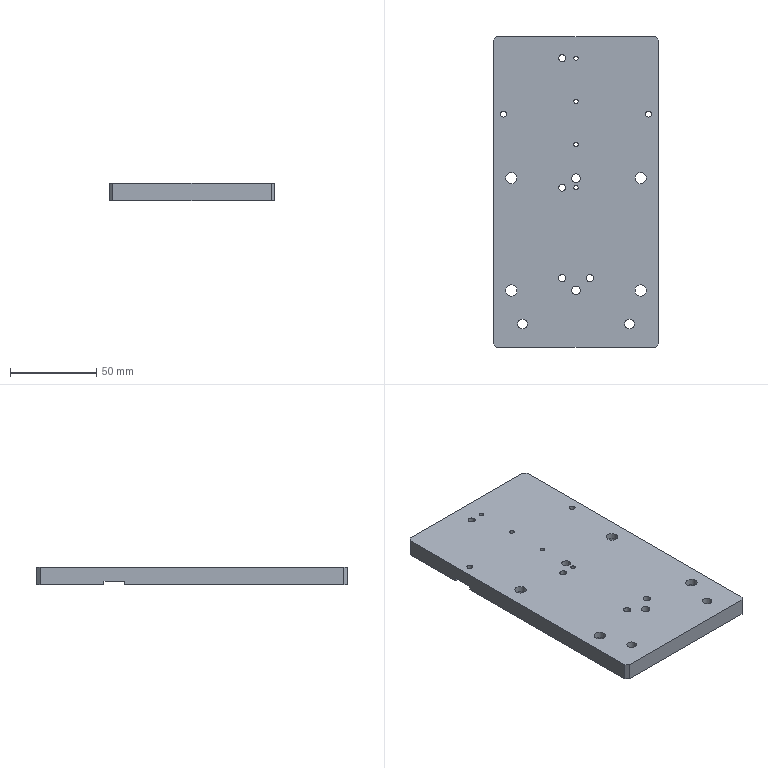CAM job | NX | 3-axis milling, drilling | part box 96 x 180 x 10 mm | stock box 101 x 185 x 12 mm
Tools:
number,name,description,diameter,corner_radius,flute_length,length,flutes
6,D6,平底铣刀-粗,6.0,0.0,25.0,75.0,2
9,D10,平底铣刀-粗,10.0,0.0,35.0,75.0,2
7,D6-J,平底铣刀-精,6.0,0.0,25.0,75.0,2
10,D10-J,平底铣刀-精,10.0,0.0,35.0,75.0,2
1,D80R0.8_FACE_MILL,圆鼻刀-粗,80.0,0.8,50.0,75.0,2
1,D80R0.8_FACE_MILL-J,圆鼻刀-精,80.0,0.8,50.0,75.0,2
2,D6_CHAMFER_MILL,倒角刀,6.0,0.0,3.0,25.0,2
20,M3X0.5,丝锥,2.5,0.0,35.0,50.0,2
21,M4X0.7,丝锥,3.3,0.0,35.0,50.0,2
22,M5X0.8,丝锥,4.2,0.0,35.0,50.0,2
24,D4_REAMER,Drilling Tool,4.0,0.0,75.0,100.0,6
11,D5_REAMER,Drilling Tool,5.0,0.0,75.0,100.0,6
12,ZT2.6,钻头,2.6,0.0,35.0,50.0,2
13,ZT3.4,钻头,3.4,0.0,35.0,50.0,2
19,ZT5.5,钻头,5.5,0.0,35.0,50.0,2
23,DRILL_6.6,Drilling Tool,6.6,0.0,35.0,50.0,2
17,ZT3.9,Drilling Tool,3.9,0.0,35.0,50.0,2
18,ZT4.9,Drilling Tool,4.9,0.0,35.0,50.0,2
14,ZT4.3,Drilling Tool,4.3,0.0,50.0,75.0,4
Operations:
program,operation,operation_type,tool,method,geometry_group,spindle_rpm,surface_speed,feed_per_tooth,feed_cut,feed_plunge,cut_length_mm,path_length_mm,cut_time_min,machine_time_min
B,FLOOR_WALL_FACE_MILL_ROUGH_COPY,VolumeBased25DMillingOperation,D80R0.8_FACE_MILL,LAYER_ROUGH-DEPTHK-STEPG,W-B,2800.0,703.696,0.5357,3000.0,100.0,2330.79,2547.673,0.7769,0.7986
B,FLOOR_WALL_FACE_MILL_FINISH_COPY,VolumeBased25DMillingOperation,D80R0.8_FACE_MILL-J,SIDE_FINISH-DEPTHK-STEPG,W-B,4000.0,1005.28,0.125,1000.0,100.0,582.11,678.11,0.5821,0.5917
B,NG_DRILL_CHAMFER_4,Operation,D6_CHAMFER_MILL,METHOD,W-B,8000.0,150.796,0.0625,1000.0,0.0,19.0,222.538,0.019,0.0394
B,NG_DRILL_CHAMFER_5,Operation,D6_CHAMFER_MILL,METHOD,W-B,8000.0,150.796,0.0625,1000.0,0.0,10.4,207.854,0.0104,0.0301
B,NG_DRILL_CHAMFER_6,Operation,D6_CHAMFER_MILL,METHOD,W-B,8000.0,150.796,0.0625,1000.0,0.0,10.6,199.26,0.0106,0.0295
B,NG_DRILL_CHAMFER_7,Operation,D6_CHAMFER_MILL,METHOD,W-B,8000.0,150.796,0.0625,1000.0,0.0,11.6,191.269,0.0116,0.0296
B,NG_DRILL_CHAMFER_8,Operation,D6_CHAMFER_MILL,METHOD,W-B,8000.0,150.796,0.0625,1000.0,0.0,11.4,142.079,0.0114,0.0245
B,MILL_CHAMFER_5,PlanarMilling,D6_CHAMFER_MILL,METHOD,W-B,8000.0,150.796,0.075,1200.0,100.0,35.589,301.203,0.0297,0.0562
B,MILL_CHAMFER_6,PlanarMilling,D6_CHAMFER_MILL,METHOD,W-B,8000.0,150.796,0.075,1200.0,100.0,81.784,694.015,0.0682,0.1294
B,C0.3_CLOSED_CONTOUR_CHAMFER_6X45L_COPY,PlanarMilling,D6_CHAMFER_MILL,WALL_CHAMFER-DEPTH0-STEPG,W-B,7000.0,131.0,0.1071,1500.0,100.0,564.842,660.842,0.3766,0.3862
A,TOP_FACE,FaceMilling,D80R0.8_FACE_MILL,SIDE_FINISH-DEPTHK-STEPG,W-A,4500.0,1385.0,0.1667,1500.0,100.0,882.0,978.0,0.588,0.5976
A,PROFILE_ROUGH_2,VolumeBased25DMillingOperation,D10,METHOD,W-A,8000.0,251.327,0.375,6000.0,80.0,8691.876,8800.376,1.449,1.46
A,FLOOR_WALL_ROUGH_1,VolumeBased25DMillingOperation,D10,METHOD,W-A,9000.0,282.743,0.3333,6000.0,100.0,832.8,1058.803,0.1388,0.1614
A,SPOT-DEPTH0.8,Operation,D6_CHAMFER_MILL,NONE,W-A,8000.0,150.796,0.0312,500.0,90.0,32.4,631.955,0.0648,0.1248
A,THROUGH_HOLE-M4_TAP_DRILL,Operation,ZT3.4,NONE,W-A,3000.0,31.102,0.05,300.0,90.0,32.0,253.006,0.1067,0.1288
A,THROUGH_HOLE-PRECISION_4.0_PREDRILL,Operation,ZT3.9,NONE,W-A,3000.0,36.757,0.0417,250.0,90.0,30.252,236.51,0.121,0.1416
A,THROUGH_HOLE-M5_TAP_DRILL,Operation,ZT4.3,NONE,W-A,3000.0,39.584,0.0583,350.0,90.0,38.0,193.031,0.1086,0.1241
A,THROUGH_HOLE-PRECISION_6.0_PREDRILL,Operation,ZT4.9,NONE,W-A,2500.0,38.484,0.05,250.0,90.0,30.829,227.666,0.1233,0.143
A,COUNTERBORE-DRILL_STAGE0,Operation,ZT5.5,NONE,W-A,1200.0,20.735,0.0625,150.0,90.0,29.305,221.618,0.1954,0.2146
A,COUNTERBORE-DRILL_STAGE0_2,Operation,DRILL_6.6,NONE,W-A,1200.0,24.881,0.0625,150.0,90.0,59.621,427.264,0.3975,0.4342
A,THROUGH_HOLE-M3_TAP_DRILL,Operation,ZT2.6,NONE,W-A,3000.0,23.562,0.05,300.0,90.0,68.0,314.06,0.2267,0.2513
A,HOLE_MILL_ROUGH_D6_1,CylinderMilling,D6,NONE,W-A,8000.0,150.796,0.075,1200.0,100.0,317.799,589.599,0.2648,0.292
A,HOLE_MILL_ROUGH_D6_2,CylinderMilling,D6,NONE,W-A,8000.0,150.796,0.075,1200.0,100.0,923.332,1551.932,0.7694,0.8323
A,HOLE_MILL_FINISH_D6_1,CylinderMilling,D6-J,FINISH_STEPDEPTH_OFF,W-A,8000.0,150.796,0.0312,500.0,100.0,66.797,339.597,0.1336,0.1609
A,HOLE_MILL_FINISH_D6_2,CylinderMilling,D6-J,FINISH_STEPDEPTH_OFF,W-A,8000.0,150.796,0.0312,500.0,100.0,178.461,809.061,0.3569,0.42
A,BODY_ONLY,SurfaceContour,D6_CHAMFER_MILL,METHOD,W-A,8000.0,150.796,0.1875,3000.0,100.0,785.717,1409.867,0.2619,0.3243
A,NG_DRILL_CHAMFER_1,Operation,D6_CHAMFER_MILL,METHOD,W-A,8000.0,150.796,0.0312,500.0,0.0,19.0,222.538,0.038,0.0584
A,NG_DRILL_CHAMFER_2,Operation,D6_CHAMFER_MILL,METHOD,W-A,8000.0,150.796,0.0312,500.0,0.0,10.4,211.854,0.0208,0.0409
A,NG_DRILL_CHAMFER_3,Operation,D6_CHAMFER_MILL,METHOD,W-A,8000.0,150.796,0.0312,500.0,0.0,10.6,199.26,0.0212,0.0401
A,MILL_CHAMFER_1,PlanarMilling,D6_CHAMFER_MILL,METHOD,W-A,8000.0,150.796,0.0312,500.0,100.0,36.041,254.101,0.0721,0.0939
A,MILL_CHAMFER_2,PlanarMilling,D6_CHAMFER_MILL,METHOD,W-A,8000.0,150.796,0.0312,500.0,100.0,36.963,305.532,0.0739,0.1008
A,MILL_CHAMFER_3,PlanarMilling,D6_CHAMFER_MILL,NONE,W-A,8000.0,150.796,0.05,800.0,100.0,80.502,327.714,0.1006,0.1253
A,MILL_CHAMFER_4,PlanarMilling,D6_CHAMFER_MILL,NONE,W-A,8000.0,150.796,0.05,800.0,100.0,173.57,770.207,0.217,0.2766
A,THROUGH_HOLE-TAP_M3,Operation,M3X0.5,METHOD,W-A,800.0,6.283,0.0003,0.5,90.0,56.0,290.06,112.0,112.023
A,THROUGH_HOLE-TAP_M4,Operation,M4X0.7,METHOD,W-A,600.0,6.22,0.0006,0.7,90.0,24.0,237.006,34.286,34.307
A,THROUGH_HOLE-TAP_M5,Operation,M5X0.8,METHOD,W-A,500.0,6.597,0.0008,0.8,90.0,29.0,175.031,36.25,36.265
A,REAMING,Operation,D4_REAMER,METHOD,W-A,500.0,6.283,0.0167,50.0,0.0,24.0,224.007,0.48,0.5
A,REAMING_2,Operation,D5_REAMER,METHOD,W-A,500.0,7.854,0.0167,50.0,0.0,24.0,214.008,0.48,0.499
A,FLOOR_SIDE_FINISH_3,VolumeBased25DMillingOperation,D10-J,METHOD,W-A,9000.0,169.646,0.0556,1000.0,100.0,217.843,320.843,0.2178,0.2281
A,PROFILE_SEMI_FINISH_2,VolumeBased25DMillingOperation,D6-J,METHOD,W-A,9000.0,169.646,0.0667,1200.0,100.0,571.08,690.08,0.4759,0.4878